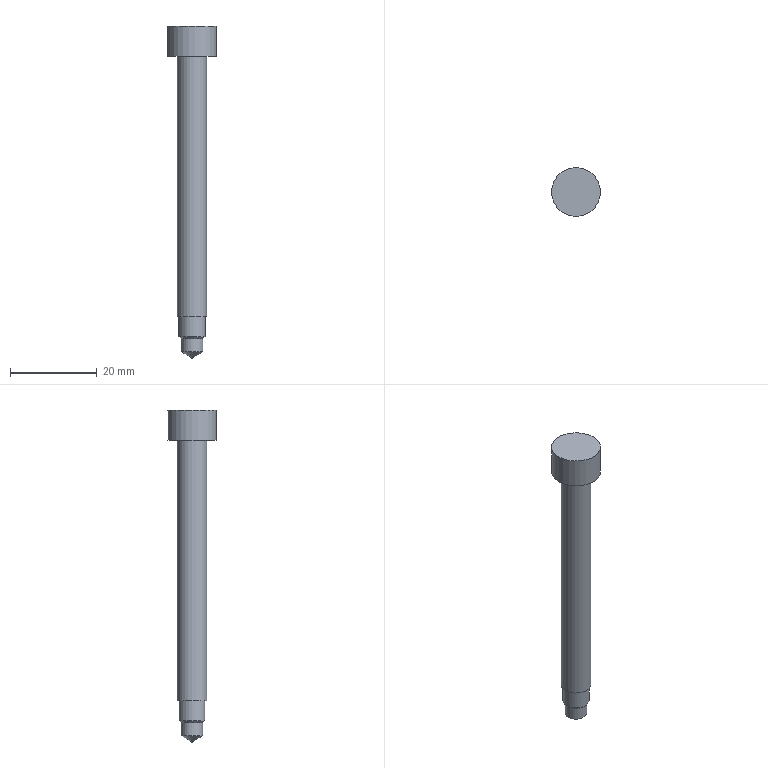Part | NX | features BREP 2 | 2 solids | 21 faces | box 11.25 x 11.25 x 76.442 mm | volume 5251 mm3 | plane 14 | cylinder 5 | cone 2 | commonest cylinder face diameters 5 x1 6 x1 6.8 x1 10 x1 11.25 x1
STEP:
#1=CARTESIAN_POINT('',(5.,0.,66.));
#2=VERTEX_POINT('',#1);
#3=CARTESIAN_POINT('',(0.,0.,66.));
#4=DIRECTION('',(0.,0.,1.));
#5=DIRECTION('',(1.,0.,0.));
#6=AXIS2_PLACEMENT_3D('',#3,#4,#5);
#7=CIRCLE('',#6,5.);
#8=EDGE_CURVE('',#2,#2,#7,.T.);
#9=ORIENTED_EDGE('',*,*,#8,.T.);
#10=EDGE_LOOP('',(#9));
#11=FACE_BOUND('',#10,.T.);
#12=CARTESIAN_POINT('',(-2.887,0.,66.));
#13=VERTEX_POINT('',#12);
#14=CARTESIAN_POINT('',(-1.443,-2.5,66.));
#15=VERTEX_POINT('',#14);
#16=CARTESIAN_POINT('',(-2.887,0.,66.));
#17=DIRECTION('',(0.5,-0.866,0.));
#18=VECTOR('',#17,1000.);
#19=LINE('',#16,#18);
#20=EDGE_CURVE('',#13,#15,#19,.T.);
#21=ORIENTED_EDGE('',*,*,#20,.F.);
#22=CARTESIAN_POINT('',(-1.443,2.5,66.));
#23=VERTEX_POINT('',#22);
#24=CARTESIAN_POINT('',(-1.443,2.5,66.));
#25=DIRECTION('',(-0.5,-0.866,0.));
#26=VECTOR('',#25,1000.);
#27=LINE('',#24,#26);
#28=EDGE_CURVE('',#23,#13,#27,.T.);
#29=ORIENTED_EDGE('',*,*,#28,.F.);
#30=CARTESIAN_POINT('',(1.443,2.5,66.));
#31=VERTEX_POINT('',#30);
#32=CARTESIAN_POINT('',(1.443,2.5,66.));
#33=DIRECTION('',(-1.,0.,0.));
#34=VECTOR('',#33,1000.);
#35=LINE('',#32,#34);
#36=EDGE_CURVE('',#31,#23,#35,.T.);
#37=ORIENTED_EDGE('',*,*,#36,.F.);
#38=CARTESIAN_POINT('',(2.887,0.,66.));
#39=VERTEX_POINT('',#38);
#40=CARTESIAN_POINT('',(2.887,0.,66.));
#41=DIRECTION('',(-0.5,0.866,0.));
#42=VECTOR('',#41,1000.);
#43=LINE('',#40,#42);
#44=EDGE_CURVE('',#39,#31,#43,.T.);
#45=ORIENTED_EDGE('',*,*,#44,.F.);
#46=CARTESIAN_POINT('',(1.443,-2.5,66.));
#47=VERTEX_POINT('',#46);
#48=CARTESIAN_POINT('',(1.443,-2.5,66.));
#49=DIRECTION('',(0.5,0.866,0.));
#50=VECTOR('',#49,1000.);
#51=LINE('',#48,#50);
#52=EDGE_CURVE('',#47,#39,#51,.T.);
#53=ORIENTED_EDGE('',*,*,#52,.F.);
#54=CARTESIAN_POINT('',(-1.443,-2.5,66.));
#55=DIRECTION('',(1.,0.,0.));
#56=VECTOR('',#55,1000.);
#57=LINE('',#54,#56);
#58=EDGE_CURVE('',#15,#47,#57,.T.);
#59=ORIENTED_EDGE('',*,*,#58,.F.);
#60=EDGE_LOOP('',(#21,#29,#37,#45,#53,#59));
#61=FACE_BOUND('',#60,.T.);
#62=CARTESIAN_POINT('',(0.,0.,66.));
#63=DIRECTION('',(0.,0.,1.));
#64=DIRECTION('',(-1.,0.,0.));
#65=AXIS2_PLACEMENT_3D('',#62,#63,#64);
#66=PLANE('',#65);
#67=ADVANCED_FACE('',(#11,#61),#66,.T.);
#68=CARTESIAN_POINT('',(3.,0.,-4.5));
#69=VERTEX_POINT('',#68);
#70=CARTESIAN_POINT('',(0.,0.,-4.5));
#71=DIRECTION('',(0.,0.,1.));
#72=DIRECTION('',(1.,0.,0.));
#73=AXIS2_PLACEMENT_3D('',#70,#71,#72);
#74=CIRCLE('',#73,3.);
#75=EDGE_CURVE('',#69,#69,#74,.T.);
#76=ORIENTED_EDGE('',*,*,#75,.T.);
#77=EDGE_LOOP('',(#76));
#78=FACE_BOUND('',#77,.T.);
#79=CARTESIAN_POINT('',(3.,0.,60.));
#80=VERTEX_POINT('',#79);
#81=CARTESIAN_POINT('',(0.,0.,60.));
#82=DIRECTION('',(0.,0.,1.));
#83=DIRECTION('',(1.,0.,0.));
#84=AXIS2_PLACEMENT_3D('',#81,#82,#83);
#85=CIRCLE('',#84,3.);
#86=EDGE_CURVE('',#80,#80,#85,.T.);
#87=ORIENTED_EDGE('',*,*,#86,.F.);
#88=EDGE_LOOP('',(#87));
#89=FACE_BOUND('',#88,.T.);
#90=CARTESIAN_POINT('',(0.,0.,60.));
#91=DIRECTION('',(0.,0.,-1.));
#92=DIRECTION('',(1.,0.,0.));
#93=AXIS2_PLACEMENT_3D('',#90,#91,#92);
#94=CYLINDRICAL_SURFACE('',#93,3.);
#95=ADVANCED_FACE('',(#78,#89),#94,.T.);
#96=CARTESIAN_POINT('',(2.5,0.,-5.));
#97=VERTEX_POINT('',#96);
#98=CARTESIAN_POINT('',(0.,0.,-5.));
#99=DIRECTION('',(0.,0.,-1.));
#100=DIRECTION('',(1.,0.,0.));
#101=AXIS2_PLACEMENT_3D('',#98,#99,#100);
#102=CIRCLE('',#101,2.5);
#103=EDGE_CURVE('',#97,#97,#102,.T.);
#104=ORIENTED_EDGE('',*,*,#103,.T.);
#105=EDGE_LOOP('',(#104));
#106=FACE_BOUND('',#105,.T.);
#107=CARTESIAN_POINT('',(0.,0.,-5.));
#108=DIRECTION('',(0.,0.,1.));
#109=DIRECTION('',(-1.,0.,0.));
#110=AXIS2_PLACEMENT_3D('',#107,#108,#109);
#111=PLANE('',#110);
#112=ADVANCED_FACE('',(#106),#111,.F.);
#113=CARTESIAN_POINT('',(5.,0.,60.));
#114=VERTEX_POINT('',#113);
#115=CARTESIAN_POINT('',(0.,0.,60.));
#116=DIRECTION('',(0.,0.,1.));
#117=DIRECTION('',(1.,0.,0.));
#118=AXIS2_PLACEMENT_3D('',#115,#116,#117);
#119=CIRCLE('',#118,5.);
#120=EDGE_CURVE('',#114,#114,#119,.T.);
#121=ORIENTED_EDGE('',*,*,#120,.F.);
#122=EDGE_LOOP('',(#121));
#123=FACE_BOUND('',#122,.T.);
#124=ORIENTED_EDGE('',*,*,#86,.T.);
#125=EDGE_LOOP('',(#124));
#126=FACE_BOUND('',#125,.T.);
#127=CARTESIAN_POINT('',(0.,0.,60.));
#128=DIRECTION('',(0.,0.,1.));
#129=DIRECTION('',(-1.,0.,0.));
#130=AXIS2_PLACEMENT_3D('',#127,#128,#129);
#131=PLANE('',#130);
#132=ADVANCED_FACE('',(#123,#126),#131,.F.);
#133=ORIENTED_EDGE('',*,*,#8,.F.);
#134=EDGE_LOOP('',(#133));
#135=FACE_BOUND('',#134,.T.);
#136=ORIENTED_EDGE('',*,*,#120,.T.);
#137=EDGE_LOOP('',(#136));
#138=FACE_BOUND('',#137,.T.);
#139=CARTESIAN_POINT('',(0.,0.,66.));
#140=DIRECTION('',(0.,0.,-1.));
#141=DIRECTION('',(1.,0.,0.));
#142=AXIS2_PLACEMENT_3D('',#139,#140,#141);
#143=CYLINDRICAL_SURFACE('',#142,5.);
#144=ADVANCED_FACE('',(#135,#138),#143,.T.);
#145=CARTESIAN_POINT('',(-1.443,2.5,61.5));
#146=VERTEX_POINT('',#145);
#147=CARTESIAN_POINT('',(-2.887,0.,61.5));
#148=VERTEX_POINT('',#147);
#149=CARTESIAN_POINT('',(-1.443,2.5,61.5));
#150=DIRECTION('',(-0.5,-0.866,0.));
#151=VECTOR('',#150,1000.);
#152=LINE('',#149,#151);
#153=EDGE_CURVE('',#146,#148,#152,.T.);
#154=ORIENTED_EDGE('',*,*,#153,.F.);
#155=CARTESIAN_POINT('',(-1.443,2.5,66.));
#156=DIRECTION('',(0.,0.,-1.));
#157=VECTOR('',#156,1000.);
#158=LINE('',#155,#157);
#159=EDGE_CURVE('',#23,#146,#158,.T.);
#160=ORIENTED_EDGE('',*,*,#159,.F.);
#161=ORIENTED_EDGE('',*,*,#28,.T.);
#162=CARTESIAN_POINT('',(-2.887,0.,66.));
#163=DIRECTION('',(0.,0.,-1.));
#164=VECTOR('',#163,1000.);
#165=LINE('',#162,#164);
#166=EDGE_CURVE('',#13,#148,#165,.T.);
#167=ORIENTED_EDGE('',*,*,#166,.T.);
#168=EDGE_LOOP('',(#154,#160,#161,#167));
#169=FACE_BOUND('',#168,.T.);
#170=CARTESIAN_POINT('',(-1.443,2.5,66.));
#171=DIRECTION('',(0.866,-0.5,0.));
#172=DIRECTION('',(-0.5,-0.866,0.));
#173=AXIS2_PLACEMENT_3D('',#170,#171,#172);
#174=PLANE('',#173);
#175=ADVANCED_FACE('',(#169),#174,.T.);
#176=CARTESIAN_POINT('',(-1.443,-2.5,61.5));
#177=VERTEX_POINT('',#176);
#178=CARTESIAN_POINT('',(-2.887,0.,61.5));
#179=DIRECTION('',(0.5,-0.866,0.));
#180=VECTOR('',#179,1000.);
#181=LINE('',#178,#180);
#182=EDGE_CURVE('',#148,#177,#181,.T.);
#183=ORIENTED_EDGE('',*,*,#182,.F.);
#184=ORIENTED_EDGE('',*,*,#166,.F.);
#185=ORIENTED_EDGE('',*,*,#20,.T.);
#186=CARTESIAN_POINT('',(-1.443,-2.5,66.));
#187=DIRECTION('',(0.,0.,-1.));
#188=VECTOR('',#187,1000.);
#189=LINE('',#186,#188);
#190=EDGE_CURVE('',#15,#177,#189,.T.);
#191=ORIENTED_EDGE('',*,*,#190,.T.);
#192=EDGE_LOOP('',(#183,#184,#185,#191));
#193=FACE_BOUND('',#192,.T.);
#194=CARTESIAN_POINT('',(-2.887,0.,66.));
#195=DIRECTION('',(0.866,0.5,0.));
#196=DIRECTION('',(0.5,-0.866,0.));
#197=AXIS2_PLACEMENT_3D('',#194,#195,#196);
#198=PLANE('',#197);
#199=ADVANCED_FACE('',(#193),#198,.T.);
#200=CARTESIAN_POINT('',(1.443,-2.5,61.5));
#201=VERTEX_POINT('',#200);
#202=CARTESIAN_POINT('',(-1.443,-2.5,61.5));
#203=DIRECTION('',(1.,0.,0.));
#204=VECTOR('',#203,1000.);
#205=LINE('',#202,#204);
#206=EDGE_CURVE('',#177,#201,#205,.T.);
#207=ORIENTED_EDGE('',*,*,#206,.F.);
#208=ORIENTED_EDGE('',*,*,#190,.F.);
#209=ORIENTED_EDGE('',*,*,#58,.T.);
#210=CARTESIAN_POINT('',(1.443,-2.5,66.));
#211=DIRECTION('',(0.,0.,-1.));
#212=VECTOR('',#211,1000.);
#213=LINE('',#210,#212);
#214=EDGE_CURVE('',#47,#201,#213,.T.);
#215=ORIENTED_EDGE('',*,*,#214,.T.);
#216=EDGE_LOOP('',(#207,#208,#209,#215));
#217=FACE_BOUND('',#216,.T.);
#218=CARTESIAN_POINT('',(-1.443,-2.5,66.));
#219=DIRECTION('',(0.,1.,0.));
#220=DIRECTION('',(0.,0.,-1.));
#221=AXIS2_PLACEMENT_3D('',#218,#219,#220);
#222=PLANE('',#221);
#223=ADVANCED_FACE('',(#217),#222,.T.);
#224=CARTESIAN_POINT('',(2.887,0.,61.5));
#225=VERTEX_POINT('',#224);
#226=CARTESIAN_POINT('',(1.443,-2.5,61.5));
#227=DIRECTION('',(0.5,0.866,0.));
#228=VECTOR('',#227,1000.);
#229=LINE('',#226,#228);
#230=EDGE_CURVE('',#201,#225,#229,.T.);
#231=ORIENTED_EDGE('',*,*,#230,.F.);
#232=ORIENTED_EDGE('',*,*,#214,.F.);
#233=ORIENTED_EDGE('',*,*,#52,.T.);
#234=CARTESIAN_POINT('',(2.887,0.,66.));
#235=DIRECTION('',(0.,0.,-1.));
#236=VECTOR('',#235,1000.);
#237=LINE('',#234,#236);
#238=EDGE_CURVE('',#39,#225,#237,.T.);
#239=ORIENTED_EDGE('',*,*,#238,.T.);
#240=EDGE_LOOP('',(#231,#232,#233,#239));
#241=FACE_BOUND('',#240,.T.);
#242=CARTESIAN_POINT('',(1.443,-2.5,66.));
#243=DIRECTION('',(-0.866,0.5,0.));
#244=DIRECTION('',(0.5,0.866,0.));
#245=AXIS2_PLACEMENT_3D('',#242,#243,#244);
#246=PLANE('',#245);
#247=ADVANCED_FACE('',(#241),#246,.T.);
#248=CARTESIAN_POINT('',(1.443,2.5,61.5));
#249=VERTEX_POINT('',#248);
#250=CARTESIAN_POINT('',(2.887,0.,61.5));
#251=DIRECTION('',(-0.5,0.866,0.));
#252=VECTOR('',#251,1000.);
#253=LINE('',#250,#252);
#254=EDGE_CURVE('',#225,#249,#253,.T.);
#255=ORIENTED_EDGE('',*,*,#254,.F.);
#256=ORIENTED_EDGE('',*,*,#238,.F.);
#257=ORIENTED_EDGE('',*,*,#44,.T.);
#258=CARTESIAN_POINT('',(1.443,2.5,66.));
#259=DIRECTION('',(0.,0.,-1.));
#260=VECTOR('',#259,1000.);
#261=LINE('',#258,#260);
#262=EDGE_CURVE('',#31,#249,#261,.T.);
#263=ORIENTED_EDGE('',*,*,#262,.T.);
#264=EDGE_LOOP('',(#255,#256,#257,#263));
#265=FACE_BOUND('',#264,.T.);
#266=CARTESIAN_POINT('',(2.887,0.,66.));
#267=DIRECTION('',(-0.866,-0.5,0.));
#268=DIRECTION('',(-0.5,0.866,0.));
#269=AXIS2_PLACEMENT_3D('',#266,#267,#268);
#270=PLANE('',#269);
#271=ADVANCED_FACE('',(#265),#270,.T.);
#272=CARTESIAN_POINT('',(1.443,2.5,61.5));
#273=DIRECTION('',(-1.,0.,0.));
#274=VECTOR('',#273,1000.);
#275=LINE('',#272,#274);
#276=EDGE_CURVE('',#249,#146,#275,.T.);
#277=ORIENTED_EDGE('',*,*,#276,.F.);
#278=ORIENTED_EDGE('',*,*,#262,.F.);
#279=ORIENTED_EDGE('',*,*,#36,.T.);
#280=ORIENTED_EDGE('',*,*,#159,.T.);
#281=EDGE_LOOP('',(#277,#278,#279,#280));
#282=FACE_BOUND('',#281,.T.);
#283=CARTESIAN_POINT('',(1.443,2.5,66.));
#284=DIRECTION('',(0.,-1.,0.));
#285=DIRECTION('',(0.,0.,1.));
#286=AXIS2_PLACEMENT_3D('',#283,#284,#285);
#287=PLANE('',#286);
#288=ADVANCED_FACE('',(#282),#287,.T.);
#289=ORIENTED_EDGE('',*,*,#153,.T.);
#290=ORIENTED_EDGE('',*,*,#182,.T.);
#291=ORIENTED_EDGE('',*,*,#206,.T.);
#292=ORIENTED_EDGE('',*,*,#230,.T.);
#293=ORIENTED_EDGE('',*,*,#254,.T.);
#294=ORIENTED_EDGE('',*,*,#276,.T.);
#295=EDGE_LOOP('',(#289,#290,#291,#292,#293,#294));
#296=FACE_BOUND('',#295,.T.);
#297=CARTESIAN_POINT('',(-2.887,0.,61.5));
#298=DIRECTION('',(0.,0.,1.));
#299=DIRECTION('',(-1.,0.,0.));
#300=AXIS2_PLACEMENT_3D('',#297,#298,#299);
#301=PLANE('',#300);
#302=ADVANCED_FACE('',(#296),#301,.T.);
#303=ORIENTED_EDGE('',*,*,#103,.F.);
#304=EDGE_LOOP('',(#303));
#305=FACE_BOUND('',#304,.T.);
#306=ORIENTED_EDGE('',*,*,#75,.F.);
#307=EDGE_LOOP('',(#306));
#308=FACE_BOUND('',#307,.T.);
#309=CARTESIAN_POINT('',(0.,0.,-4.5));
#310=DIRECTION('',(0.,0.,1.));
#311=DIRECTION('',(-1.,0.,0.));
#312=AXIS2_PLACEMENT_3D('',#309,#310,#311);
#313=CONICAL_SURFACE('',#312,3.,0.7854);
#314=ADVANCED_FACE('',(#305,#308),#313,.T.);
#315=CLOSED_SHELL('',(#67,#95,#112,#132,#144,#175,#199,#223,#247,#271,#288,#302,#314));
#316=MANIFOLD_SOLID_BREP('',#315);
#317=CARTESIAN_POINT('',(3.4,0.,60.));
#318=VERTEX_POINT('',#317);
#319=CARTESIAN_POINT('',(0.,0.,60.));
#320=DIRECTION('',(0.,0.,1.));
#321=DIRECTION('',(1.,0.,0.));
#322=AXIS2_PLACEMENT_3D('',#319,#320,#321);
#323=CIRCLE('',#322,3.4);
#324=EDGE_CURVE('',#318,#318,#323,.T.);
#325=ORIENTED_EDGE('',*,*,#324,.F.);
#326=EDGE_LOOP('',(#325));
#327=FACE_BOUND('',#326,.T.);
#328=CARTESIAN_POINT('',(3.4,0.,0.));
#329=VERTEX_POINT('',#328);
#330=CARTESIAN_POINT('',(0.,0.,0.));
#331=DIRECTION('',(0.,0.,1.));
#332=DIRECTION('',(1.,0.,0.));
#333=AXIS2_PLACEMENT_3D('',#330,#331,#332);
#334=CIRCLE('',#333,3.4);
#335=EDGE_CURVE('',#329,#329,#334,.T.);
#336=ORIENTED_EDGE('',*,*,#335,.T.);
#337=EDGE_LOOP('',(#336));
#338=FACE_BOUND('',#337,.T.);
#339=CARTESIAN_POINT('',(0.,0.,60.));
#340=DIRECTION('',(0.,0.,-1.));
#341=DIRECTION('',(1.,0.,0.));
#342=AXIS2_PLACEMENT_3D('',#339,#340,#341);
#343=CYLINDRICAL_SURFACE('',#342,3.4);
#344=ADVANCED_FACE('',(#327,#338),#343,.T.);
#345=CARTESIAN_POINT('',(2.5,0.,0.));
#346=VERTEX_POINT('',#345);
#347=CARTESIAN_POINT('',(0.,0.,0.));
#348=DIRECTION('',(0.,0.,1.));
#349=DIRECTION('',(1.,0.,0.));
#350=AXIS2_PLACEMENT_3D('',#347,#348,#349);
#351=CIRCLE('',#350,2.5);
#352=EDGE_CURVE('',#346,#346,#351,.T.);
#353=ORIENTED_EDGE('',*,*,#352,.T.);
#354=EDGE_LOOP('',(#353));
#355=FACE_BOUND('',#354,.T.);
#356=ORIENTED_EDGE('',*,*,#335,.F.);
#357=EDGE_LOOP('',(#356));
#358=FACE_BOUND('',#357,.T.);
#359=CARTESIAN_POINT('',(0.,0.,0.));
#360=DIRECTION('',(0.,0.,1.));
#361=DIRECTION('',(-1.,0.,0.));
#362=AXIS2_PLACEMENT_3D('',#359,#360,#361);
#363=PLANE('',#362);
#364=ADVANCED_FACE('',(#355,#358),#363,.F.);
#365=CARTESIAN_POINT('',(5.625,0.,60.));
#366=VERTEX_POINT('',#365);
#367=CARTESIAN_POINT('',(0.,0.,60.));
#368=DIRECTION('',(0.,0.,1.));
#369=DIRECTION('',(1.,0.,0.));
#370=AXIS2_PLACEMENT_3D('',#367,#368,#369);
#371=CIRCLE('',#370,5.625);
#372=EDGE_CURVE('',#366,#366,#371,.T.);
#373=ORIENTED_EDGE('',*,*,#372,.F.);
#374=EDGE_LOOP('',(#373));
#375=FACE_BOUND('',#374,.T.);
#376=ORIENTED_EDGE('',*,*,#324,.T.);
#377=EDGE_LOOP('',(#376));
#378=FACE_BOUND('',#377,.T.);
#379=CARTESIAN_POINT('',(0.,0.,60.));
#380=DIRECTION('',(0.,0.,1.));
#381=DIRECTION('',(-1.,0.,0.));
#382=AXIS2_PLACEMENT_3D('',#379,#380,#381);
#383=PLANE('',#382);
#384=ADVANCED_FACE('',(#375,#378),#383,.F.);
#385=CARTESIAN_POINT('',(5.625,0.,67.));
#386=VERTEX_POINT('',#385);
#387=CARTESIAN_POINT('',(0.,0.,67.));
#388=DIRECTION('',(0.,0.,1.));
#389=DIRECTION('',(1.,0.,0.));
#390=AXIS2_PLACEMENT_3D('',#387,#388,#389);
#391=CIRCLE('',#390,5.625);
#392=EDGE_CURVE('',#386,#386,#391,.T.);
#393=ORIENTED_EDGE('',*,*,#392,.F.);
#394=EDGE_LOOP('',(#393));
#395=FACE_BOUND('',#394,.T.);
#396=ORIENTED_EDGE('',*,*,#372,.T.);
#397=EDGE_LOOP('',(#396));
#398=FACE_BOUND('',#397,.T.);
#399=CARTESIAN_POINT('',(0.,0.,67.));
#400=DIRECTION('',(0.,0.,-1.));
#401=DIRECTION('',(1.,0.,0.));
#402=AXIS2_PLACEMENT_3D('',#399,#400,#401);
#403=CYLINDRICAL_SURFACE('',#402,5.625);
#404=ADVANCED_FACE('',(#395,#398),#403,.T.);
#405=ORIENTED_EDGE('',*,*,#392,.T.);
#406=EDGE_LOOP('',(#405));
#407=FACE_BOUND('',#406,.T.);
#408=CARTESIAN_POINT('',(0.,0.,67.));
#409=DIRECTION('',(0.,0.,1.));
#410=DIRECTION('',(-1.,0.,0.));
#411=AXIS2_PLACEMENT_3D('',#408,#409,#410);
#412=PLANE('',#411);
#413=ADVANCED_FACE('',(#407),#412,.T.);
#414=CARTESIAN_POINT('',(2.5,0.,-8.));
#415=VERTEX_POINT('',#414);
#416=CARTESIAN_POINT('',(0.,0.,-8.));
#417=DIRECTION('',(0.,0.,1.));
#418=DIRECTION('',(1.,0.,0.));
#419=AXIS2_PLACEMENT_3D('',#416,#417,#418);
#420=CIRCLE('',#419,2.5);
#421=EDGE_CURVE('',#415,#415,#420,.T.);
#422=ORIENTED_EDGE('',*,*,#421,.T.);
#423=EDGE_LOOP('',(#422));
#424=FACE_BOUND('',#423,.T.);
#425=ORIENTED_EDGE('',*,*,#352,.F.);
#426=EDGE_LOOP('',(#425));
#427=FACE_BOUND('',#426,.T.);
#428=CARTESIAN_POINT('',(0.,0.,-8.));
#429=DIRECTION('',(0.,0.,1.));
#430=DIRECTION('',(-1.,0.,0.));
#431=AXIS2_PLACEMENT_3D('',#428,#429,#430);
#432=CYLINDRICAL_SURFACE('',#431,2.5);
#433=ADVANCED_FACE('',(#424,#427),#432,.T.);
#434=CARTESIAN_POINT('',(0.001732,0.,-9.442));
#435=VERTEX_POINT('',#434);
#436=CARTESIAN_POINT('',(0.,0.,-9.442));
#437=DIRECTION('',(0.,0.,1.));
#438=DIRECTION('',(1.,0.,0.));
#439=AXIS2_PLACEMENT_3D('',#436,#437,#438);
#440=CIRCLE('',#439,0.001732);
#441=EDGE_CURVE('',#435,#435,#440,.T.);
#442=ORIENTED_EDGE('',*,*,#441,.T.);
#443=EDGE_LOOP('',(#442));
#444=FACE_BOUND('',#443,.T.);
#445=ORIENTED_EDGE('',*,*,#421,.F.);
#446=EDGE_LOOP('',(#445));
#447=FACE_BOUND('',#446,.T.);
#448=CARTESIAN_POINT('',(0.,0.,-8.));
#449=DIRECTION('',(0.,0.,1.));
#450=DIRECTION('',(1.,0.,0.));
#451=AXIS2_PLACEMENT_3D('',#448,#449,#450);
#452=CONICAL_SURFACE('',#451,2.5,1.047);
#453=ADVANCED_FACE('',(#444,#447),#452,.T.);
#454=ORIENTED_EDGE('',*,*,#441,.F.);
#455=EDGE_LOOP('',(#454));
#456=FACE_BOUND('',#455,.T.);
#457=CARTESIAN_POINT('',(0.,0.,-9.442));
#458=DIRECTION('',(0.,0.,1.));
#459=DIRECTION('',(-1.,0.,0.));
#460=AXIS2_PLACEMENT_3D('',#457,#458,#459);
#461=PLANE('',#460);
#462=ADVANCED_FACE('',(#456),#461,.F.);
#463=CLOSED_SHELL('',(#344,#364,#384,#404,#413,#433,#453,#462));
#464=MANIFOLD_SOLID_BREP('',#463);
#465=(LENGTH_UNIT()NAMED_UNIT(*)SI_UNIT(.MILLI.,.METRE.));
#466=UNCERTAINTY_MEASURE_WITH_UNIT(LENGTH_MEASURE(0.00001),#465,'','');
#467=(NAMED_UNIT(*)PLANE_ANGLE_UNIT()SI_UNIT($,.RADIAN.));
#468=(NAMED_UNIT(*)SI_UNIT($,.STERADIAN.)SOLID_ANGLE_UNIT());
#469=(GEOMETRIC_REPRESENTATION_CONTEXT(3)GLOBAL_UNCERTAINTY_ASSIGNED_CONTEXT((#466))GLOBAL_UNIT_ASSIGNED_CONTEXT((#465,#467,#468))REPRESENTATION_CONTEXT('',''));
#470=ADVANCED_BREP_SHAPE_REPRESENTATION('',(#316,#464),#469);